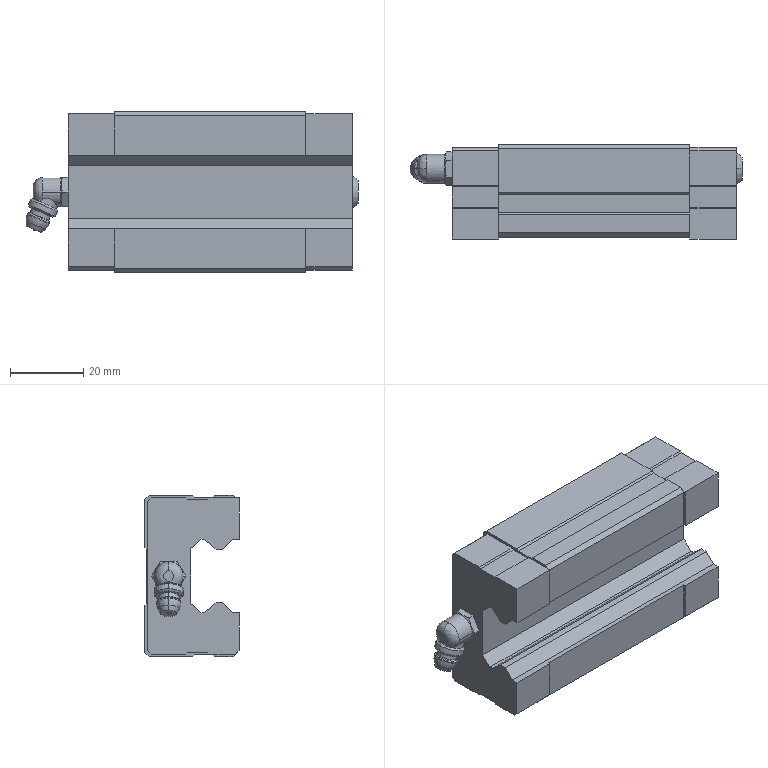Part | SolidWorks | features BaseBody 1 | 1 solid | 142 faces | box 90.473 x 25.7 x 44 mm | volume 66840 mm3 | plane 95 | cylinder 20 | cone 16 | spline 6 | torus 4 | sphere 1 | commonest cylinder face diameters 4.134 x8 7 x4 5.5 x2 6.6 x2 7.85 x2 8 x2